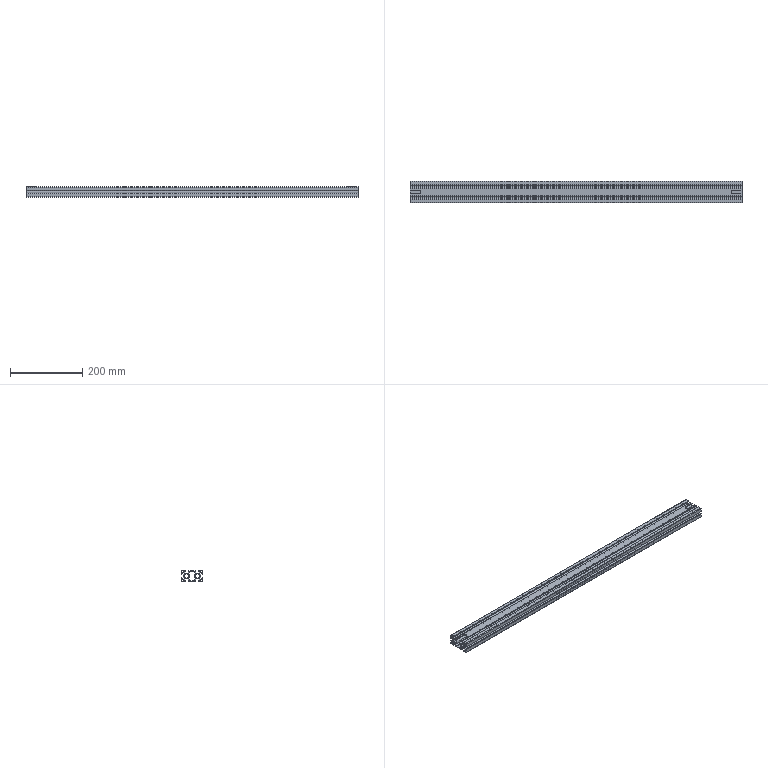Part | STEP file | belt line support ET profile 920 | 1 solid | 166 faces | box 920 x 60 x 30 mm | volume 594868 mm3 | plane 88 | cylinder 70 | cone 8 | commonest cylinder face diameters 2 x26 16 x14 1 x10 12 x8 3 x4 10 x4